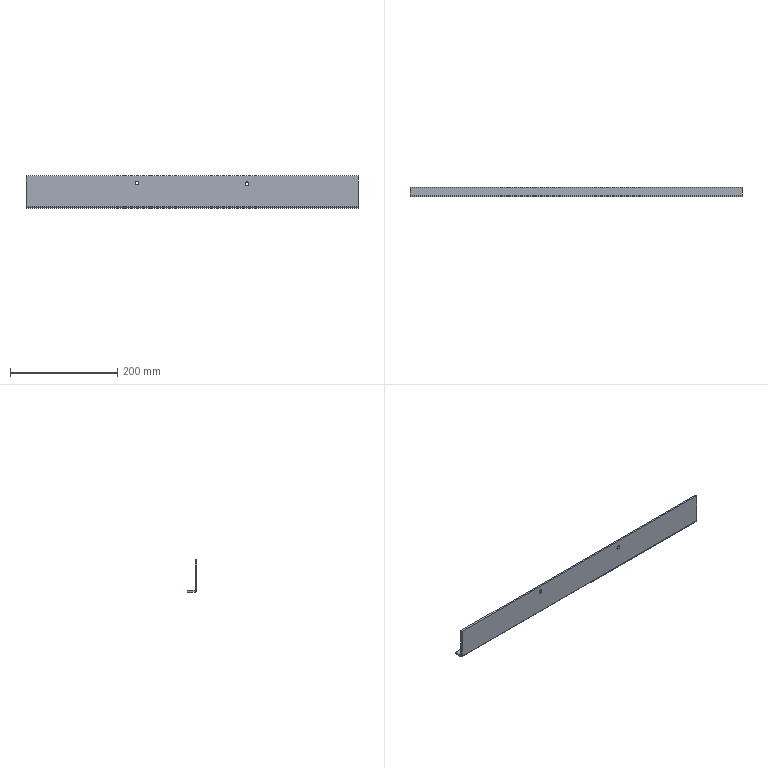Part | STEP file | HESS-408-70-15W-W-48-outer case reinforcing rib 7 | 1 solid | 14 faces | box 620 x 18 x 60 mm | volume 138005 mm3 | plane 8 | cylinder 6 | commonest cylinder face diameters 6.8 x4 0.2 x1 6.2 x1
STEP:
#1=CARTESIAN_POINT('',(0.,0.,0.));
#2=DIRECTION('',(0.,0.,1.));
#3=DIRECTION('',(1.,0.,0.));
#4=AXIS2_PLACEMENT_3D('',#1,#2,#3);
#5=CARTESIAN_POINT('',(102.5,0.,12.1));
#6=VERTEX_POINT('',#5);
#7=CARTESIAN_POINT('',(102.5,-3.,12.1));
#8=VERTEX_POINT('',#7);
#9=CARTESIAN_POINT('',(102.5,7.,12.1));
#10=DIRECTION('',(0.,-1.,0.));
#11=VECTOR('',#10,1.);
#12=LINE('',#9,#11);
#13=CARTESIAN_POINT('',(102.5,7.,15.5));
#14=DIRECTION('',(0.,-1.,0.));
#15=DIRECTION('',(0.,0.,-1.));
#16=AXIS2_PLACEMENT_3D('',#13,#14,#15);
#17=CYLINDRICAL_SURFACE('',#16,3.4);
#18=CARTESIAN_POINT('',(6.283,0.));
#19=DIRECTION('',(0.,1.));
#20=VECTOR('',#19,1.);
#21=LINE('',#18,#20);
#22=(GEOMETRIC_REPRESENTATION_CONTEXT(2)PARAMETRIC_REPRESENTATION_CONTEXT()REPRESENTATION_CONTEXT('',''));
#23=DEFINITIONAL_REPRESENTATION('',(#21),#22);
#24=PCURVE('',#17,#23);
#25=CARTESIAN_POINT('',(102.5,7.,15.5));
#26=DIRECTION('',(0.,-1.,0.));
#27=DIRECTION('',(0.,0.,-1.));
#28=AXIS2_PLACEMENT_3D('',#25,#26,#27);
#29=CYLINDRICAL_SURFACE('',#28,3.4);
#30=CARTESIAN_POINT('',(0.,0.));
#31=DIRECTION('',(0.,1.));
#32=VECTOR('',#31,1.);
#33=LINE('',#30,#32);
#34=(GEOMETRIC_REPRESENTATION_CONTEXT(2)PARAMETRIC_REPRESENTATION_CONTEXT()REPRESENTATION_CONTEXT('',''));
#35=DEFINITIONAL_REPRESENTATION('',(#33),#34);
#36=PCURVE('',#29,#35);
#37=SURFACE_CURVE('',#12,(#24,#36),.PCURVE_S1.);
#38=EDGE_CURVE('',#6,#8,#37,.T.);
#39=ORIENTED_EDGE('',*,*,#38,.T.);
#40=CARTESIAN_POINT('',(102.5,-3.,18.9));
#41=VERTEX_POINT('',#40);
#42=CARTESIAN_POINT('',(102.5,-3.,15.5));
#43=DIRECTION('',(0.,1.,0.));
#44=DIRECTION('',(0.,0.,-1.));
#45=AXIS2_PLACEMENT_3D('',#42,#43,#44);
#46=CIRCLE('',#45,3.4);
#47=CARTESIAN_POINT('',(6.283,10.));
#48=DIRECTION('',(-1.,0.));
#49=VECTOR('',#48,1.);
#50=LINE('',#47,#49);
#51=(GEOMETRIC_REPRESENTATION_CONTEXT(2)PARAMETRIC_REPRESENTATION_CONTEXT()REPRESENTATION_CONTEXT('',''));
#52=DEFINITIONAL_REPRESENTATION('',(#50),#51);
#53=PCURVE('',#17,#52);
#54=CARTESIAN_POINT('',(0.,-3.,0.));
#55=DIRECTION('',(0.,-1.,0.));
#56=DIRECTION('',(0.,0.,-1.));
#57=AXIS2_PLACEMENT_3D('',#54,#55,#56);
#58=PLANE('',#57);
#59=CARTESIAN_POINT('',(-12.1,102.5));
#60=CARTESIAN_POINT('',(-12.1,96.611));
#61=CARTESIAN_POINT('',(-17.2,99.556));
#62=CARTESIAN_POINT('',(-22.3,102.5));
#63=CARTESIAN_POINT('',(-17.2,105.444));
#64=CARTESIAN_POINT('',(-12.1,108.389));
#65=CARTESIAN_POINT('',(-12.1,102.5));
#66=(BOUNDED_CURVE()B_SPLINE_CURVE(2,(#59,#60,#61,#62,#63,#64,#65),.UNSPECIFIED.,.T.,.F.)B_SPLINE_CURVE_WITH_KNOTS((1,2,2,2,2,1),(-2.094,0.,2.094,4.189,6.283,8.378),.UNSPECIFIED.)CURVE()GEOMETRIC_REPRESENTATION_ITEM()RATIONAL_B_SPLINE_CURVE((1.,0.5,1.,0.5,1.,0.5,1.))REPRESENTATION_ITEM(''));
#67=(GEOMETRIC_REPRESENTATION_CONTEXT(2)PARAMETRIC_REPRESENTATION_CONTEXT()REPRESENTATION_CONTEXT('',''));
#68=DEFINITIONAL_REPRESENTATION('',(#66),#67);
#69=PCURVE('',#58,#68);
#70=SURFACE_CURVE('',#46,(#53,#69),.PCURVE_S1.);
#71=EDGE_CURVE('',#8,#41,#70,.T.);
#72=ORIENTED_EDGE('',*,*,#71,.T.);
#73=CARTESIAN_POINT('',(102.5,0.,18.9));
#74=VERTEX_POINT('',#73);
#75=CARTESIAN_POINT('',(102.5,7.,18.9));
#76=DIRECTION('',(0.,-1.,0.));
#77=VECTOR('',#76,1.);
#78=LINE('',#75,#77);
#79=CARTESIAN_POINT('',(3.142,0.));
#80=DIRECTION('',(0.,1.));
#81=VECTOR('',#80,1.);
#82=LINE('',#79,#81);
#83=(GEOMETRIC_REPRESENTATION_CONTEXT(2)PARAMETRIC_REPRESENTATION_CONTEXT()REPRESENTATION_CONTEXT('',''));
#84=DEFINITIONAL_REPRESENTATION('',(#82),#83);
#85=PCURVE('',#17,#84);
#86=CARTESIAN_POINT('',(3.142,0.));
#87=DIRECTION('',(0.,1.));
#88=VECTOR('',#87,1.);
#89=LINE('',#86,#88);
#90=(GEOMETRIC_REPRESENTATION_CONTEXT(2)PARAMETRIC_REPRESENTATION_CONTEXT()REPRESENTATION_CONTEXT('',''));
#91=DEFINITIONAL_REPRESENTATION('',(#89),#90);
#92=PCURVE('',#29,#91);
#93=SURFACE_CURVE('',#78,(#85,#92),.PCURVE_S1.);
#94=EDGE_CURVE('',#74,#41,#93,.T.);
#95=ORIENTED_EDGE('',*,*,#94,.F.);
#96=CARTESIAN_POINT('',(102.5,0.,15.5));
#97=DIRECTION('',(0.,-1.,0.));
#98=DIRECTION('',(0.,0.,-1.));
#99=AXIS2_PLACEMENT_3D('',#96,#97,#98);
#100=CIRCLE('',#99,3.4);
#101=CARTESIAN_POINT('',(0.,7.));
#102=DIRECTION('',(1.,0.));
#103=VECTOR('',#102,1.);
#104=LINE('',#101,#103);
#105=(GEOMETRIC_REPRESENTATION_CONTEXT(2)PARAMETRIC_REPRESENTATION_CONTEXT()REPRESENTATION_CONTEXT('',''));
#106=DEFINITIONAL_REPRESENTATION('',(#104),#105);
#107=PCURVE('',#17,#106);
#108=CARTESIAN_POINT('',(0.,0.,0.));
#109=DIRECTION('',(0.,-1.,0.));
#110=DIRECTION('',(0.,0.,-1.));
#111=AXIS2_PLACEMENT_3D('',#108,#109,#110);
#112=PLANE('',#111);
#113=CARTESIAN_POINT('',(-15.5,102.5));
#114=DIRECTION('',(1.,0.));
#115=AXIS2_PLACEMENT_2D('',#113,#114);
#116=CIRCLE('',#115,3.4);
#117=(GEOMETRIC_REPRESENTATION_CONTEXT(2)PARAMETRIC_REPRESENTATION_CONTEXT()REPRESENTATION_CONTEXT('',''));
#118=DEFINITIONAL_REPRESENTATION('',(#116),#117);
#119=PCURVE('',#112,#118);
#120=SURFACE_CURVE('',#100,(#107,#119),.PCURVE_S1.);
#121=EDGE_CURVE('',#74,#6,#120,.T.);
#122=ORIENTED_EDGE('',*,*,#121,.T.);
#123=EDGE_LOOP('',(#39,#72,#95,#122));
#124=FACE_BOUND('',#123,.F.);
#125=ADVANCED_FACE('',(#124),#17,.F.);
#126=CARTESIAN_POINT('',(-102.5,0.,13.6));
#127=VERTEX_POINT('',#126);
#128=CARTESIAN_POINT('',(-102.5,-3.,13.6));
#129=VERTEX_POINT('',#128);
#130=CARTESIAN_POINT('',(-102.5,7.,13.6));
#131=DIRECTION('',(0.,-1.,0.));
#132=VECTOR('',#131,1.);
#133=LINE('',#130,#132);
#134=CARTESIAN_POINT('',(-102.5,7.,17.));
#135=DIRECTION('',(0.,-1.,0.));
#136=DIRECTION('',(0.,0.,-1.));
#137=AXIS2_PLACEMENT_3D('',#134,#135,#136);
#138=CYLINDRICAL_SURFACE('',#137,3.4);
#139=CARTESIAN_POINT('',(6.283,0.));
#140=DIRECTION('',(0.,1.));
#141=VECTOR('',#140,1.);
#142=LINE('',#139,#141);
#143=(GEOMETRIC_REPRESENTATION_CONTEXT(2)PARAMETRIC_REPRESENTATION_CONTEXT()REPRESENTATION_CONTEXT('',''));
#144=DEFINITIONAL_REPRESENTATION('',(#142),#143);
#145=PCURVE('',#138,#144);
#146=CARTESIAN_POINT('',(-102.5,7.,17.));
#147=DIRECTION('',(0.,-1.,0.));
#148=DIRECTION('',(0.,0.,-1.));
#149=AXIS2_PLACEMENT_3D('',#146,#147,#148);
#150=CYLINDRICAL_SURFACE('',#149,3.4);
#151=CARTESIAN_POINT('',(0.,0.));
#152=DIRECTION('',(0.,1.));
#153=VECTOR('',#152,1.);
#154=LINE('',#151,#153);
#155=(GEOMETRIC_REPRESENTATION_CONTEXT(2)PARAMETRIC_REPRESENTATION_CONTEXT()REPRESENTATION_CONTEXT('',''));
#156=DEFINITIONAL_REPRESENTATION('',(#154),#155);
#157=PCURVE('',#150,#156);
#158=SURFACE_CURVE('',#133,(#145,#157),.PCURVE_S1.);
#159=EDGE_CURVE('',#127,#129,#158,.T.);
#160=ORIENTED_EDGE('',*,*,#159,.T.);
#161=CARTESIAN_POINT('',(-102.5,-3.,20.4));
#162=VERTEX_POINT('',#161);
#163=CARTESIAN_POINT('',(-102.5,-3.,17.));
#164=DIRECTION('',(0.,1.,0.));
#165=DIRECTION('',(0.,0.,-1.));
#166=AXIS2_PLACEMENT_3D('',#163,#164,#165);
#167=CIRCLE('',#166,3.4);
#168=CARTESIAN_POINT('',(6.283,10.));
#169=DIRECTION('',(-1.,0.));
#170=VECTOR('',#169,1.);
#171=LINE('',#168,#170);
#172=(GEOMETRIC_REPRESENTATION_CONTEXT(2)PARAMETRIC_REPRESENTATION_CONTEXT()REPRESENTATION_CONTEXT('',''));
#173=DEFINITIONAL_REPRESENTATION('',(#171),#172);
#174=PCURVE('',#138,#173);
#175=CARTESIAN_POINT('',(-13.6,-102.5));
#176=CARTESIAN_POINT('',(-13.6,-108.389));
#177=CARTESIAN_POINT('',(-18.7,-105.444));
#178=CARTESIAN_POINT('',(-23.8,-102.5));
#179=CARTESIAN_POINT('',(-18.7,-99.556));
#180=CARTESIAN_POINT('',(-13.6,-96.611));
#181=CARTESIAN_POINT('',(-13.6,-102.5));
#182=(BOUNDED_CURVE()B_SPLINE_CURVE(2,(#175,#176,#177,#178,#179,#180,#181),.UNSPECIFIED.,.T.,.F.)B_SPLINE_CURVE_WITH_KNOTS((1,2,2,2,2,1),(-2.094,0.,2.094,4.189,6.283,8.378),.UNSPECIFIED.)CURVE()GEOMETRIC_REPRESENTATION_ITEM()RATIONAL_B_SPLINE_CURVE((1.,0.5,1.,0.5,1.,0.5,1.))REPRESENTATION_ITEM(''));
#183=(GEOMETRIC_REPRESENTATION_CONTEXT(2)PARAMETRIC_REPRESENTATION_CONTEXT()REPRESENTATION_CONTEXT('',''));
#184=DEFINITIONAL_REPRESENTATION('',(#182),#183);
#185=PCURVE('',#58,#184);
#186=SURFACE_CURVE('',#167,(#174,#185),.PCURVE_S1.);
#187=EDGE_CURVE('',#129,#162,#186,.T.);
#188=ORIENTED_EDGE('',*,*,#187,.T.);
#189=CARTESIAN_POINT('',(-102.5,0.,20.4));
#190=VERTEX_POINT('',#189);
#191=CARTESIAN_POINT('',(-102.5,7.,20.4));
#192=DIRECTION('',(0.,-1.,0.));
#193=VECTOR('',#192,1.);
#194=LINE('',#191,#193);
#195=CARTESIAN_POINT('',(3.142,0.));
#196=DIRECTION('',(0.,1.));
#197=VECTOR('',#196,1.);
#198=LINE('',#195,#197);
#199=(GEOMETRIC_REPRESENTATION_CONTEXT(2)PARAMETRIC_REPRESENTATION_CONTEXT()REPRESENTATION_CONTEXT('',''));
#200=DEFINITIONAL_REPRESENTATION('',(#198),#199);
#201=PCURVE('',#138,#200);
#202=CARTESIAN_POINT('',(3.142,0.));
#203=DIRECTION('',(0.,1.));
#204=VECTOR('',#203,1.);
#205=LINE('',#202,#204);
#206=(GEOMETRIC_REPRESENTATION_CONTEXT(2)PARAMETRIC_REPRESENTATION_CONTEXT()REPRESENTATION_CONTEXT('',''));
#207=DEFINITIONAL_REPRESENTATION('',(#205),#206);
#208=PCURVE('',#150,#207);
#209=SURFACE_CURVE('',#194,(#201,#208),.PCURVE_S1.);
#210=EDGE_CURVE('',#190,#162,#209,.T.);
#211=ORIENTED_EDGE('',*,*,#210,.F.);
#212=CARTESIAN_POINT('',(-102.5,0.,17.));
#213=DIRECTION('',(0.,-1.,0.));
#214=DIRECTION('',(0.,0.,-1.));
#215=AXIS2_PLACEMENT_3D('',#212,#213,#214);
#216=CIRCLE('',#215,3.4);
#217=CARTESIAN_POINT('',(0.,7.));
#218=DIRECTION('',(1.,0.));
#219=VECTOR('',#218,1.);
#220=LINE('',#217,#219);
#221=(GEOMETRIC_REPRESENTATION_CONTEXT(2)PARAMETRIC_REPRESENTATION_CONTEXT()REPRESENTATION_CONTEXT('',''));
#222=DEFINITIONAL_REPRESENTATION('',(#220),#221);
#223=PCURVE('',#138,#222);
#224=CARTESIAN_POINT('',(-17.,-102.5));
#225=DIRECTION('',(1.,0.));
#226=AXIS2_PLACEMENT_2D('',#224,#225);
#227=CIRCLE('',#226,3.4);
#228=(GEOMETRIC_REPRESENTATION_CONTEXT(2)PARAMETRIC_REPRESENTATION_CONTEXT()REPRESENTATION_CONTEXT('',''));
#229=DEFINITIONAL_REPRESENTATION('',(#227),#228);
#230=PCURVE('',#112,#229);
#231=SURFACE_CURVE('',#216,(#223,#230),.PCURVE_S1.);
#232=EDGE_CURVE('',#190,#127,#231,.T.);
#233=ORIENTED_EDGE('',*,*,#232,.T.);
#234=EDGE_LOOP('',(#160,#188,#211,#233));
#235=FACE_BOUND('',#234,.F.);
#236=ADVANCED_FACE('',(#235),#138,.F.);
#237=CARTESIAN_POINT('',(310.,-3.,-26.9));
#238=VERTEX_POINT('',#237);
#239=CARTESIAN_POINT('',(310.,-3.,30.));
#240=VERTEX_POINT('',#239);
#241=CARTESIAN_POINT('',(310.,-3.,0.));
#242=DIRECTION('',(0.,0.,1.));
#243=VECTOR('',#242,1.);
#244=LINE('',#241,#243);
#245=CARTESIAN_POINT('',(0.,310.));
#246=DIRECTION('',(-1.,0.));
#247=VECTOR('',#246,1.);
#248=LINE('',#245,#247);
#249=(GEOMETRIC_REPRESENTATION_CONTEXT(2)PARAMETRIC_REPRESENTATION_CONTEXT()REPRESENTATION_CONTEXT('',''));
#250=DEFINITIONAL_REPRESENTATION('',(#248),#249);
#251=PCURVE('',#58,#250);
#252=CARTESIAN_POINT('',(310.,-3.,30.));
#253=DIRECTION('',(1.,0.,0.));
#254=DIRECTION('',(0.,0.,-1.));
#255=AXIS2_PLACEMENT_3D('',#252,#253,#254);
#256=PLANE('',#255);
#257=CARTESIAN_POINT('',(30.,0.));
#258=DIRECTION('',(-1.,0.));
#259=VECTOR('',#258,1.);
#260=LINE('',#257,#259);
#261=(GEOMETRIC_REPRESENTATION_CONTEXT(2)PARAMETRIC_REPRESENTATION_CONTEXT()REPRESENTATION_CONTEXT('',''));
#262=DEFINITIONAL_REPRESENTATION('',(#260),#261);
#263=PCURVE('',#256,#262);
#264=SURFACE_CURVE('',#244,(#251,#263),.PCURVE_S1.);
#265=EDGE_CURVE('',#238,#240,#264,.T.);
#266=ORIENTED_EDGE('',*,*,#265,.T.);
#267=CARTESIAN_POINT('',(-310.,-3.,30.));
#268=VERTEX_POINT('',#267);
#269=CARTESIAN_POINT('',(0.,-3.,30.));
#270=DIRECTION('',(-1.,0.,0.));
#271=VECTOR('',#270,1.);
#272=LINE('',#269,#271);
#273=CARTESIAN_POINT('',(-30.,0.));
#274=DIRECTION('',(0.,-1.));
#275=VECTOR('',#274,1.);
#276=LINE('',#273,#275);
#277=(GEOMETRIC_REPRESENTATION_CONTEXT(2)PARAMETRIC_REPRESENTATION_CONTEXT()REPRESENTATION_CONTEXT('',''));
#278=DEFINITIONAL_REPRESENTATION('',(#276),#277);
#279=PCURVE('',#58,#278);
#280=CARTESIAN_POINT('',(-310.,-3.,30.));
#281=DIRECTION('',(0.,0.,1.));
#282=DIRECTION('',(1.,0.,0.));
#283=AXIS2_PLACEMENT_3D('',#280,#281,#282);
#284=PLANE('',#283);
#285=CARTESIAN_POINT('',(310.,0.));
#286=DIRECTION('',(-1.,0.));
#287=VECTOR('',#286,1.);
#288=LINE('',#285,#287);
#289=(GEOMETRIC_REPRESENTATION_CONTEXT(2)PARAMETRIC_REPRESENTATION_CONTEXT()REPRESENTATION_CONTEXT('',''));
#290=DEFINITIONAL_REPRESENTATION('',(#288),#289);
#291=PCURVE('',#284,#290);
#292=SURFACE_CURVE('',#272,(#279,#291),.PCURVE_S1.);
#293=EDGE_CURVE('',#240,#268,#292,.T.);
#294=ORIENTED_EDGE('',*,*,#293,.T.);
#295=CARTESIAN_POINT('',(-310.,-3.,-26.9));
#296=VERTEX_POINT('',#295);
#297=CARTESIAN_POINT('',(-310.,-3.,0.));
#298=DIRECTION('',(0.,0.,-1.));
#299=VECTOR('',#298,1.);
#300=LINE('',#297,#299);
#301=CARTESIAN_POINT('',(0.,-310.));
#302=DIRECTION('',(1.,0.));
#303=VECTOR('',#302,1.);
#304=LINE('',#301,#303);
#305=(GEOMETRIC_REPRESENTATION_CONTEXT(2)PARAMETRIC_REPRESENTATION_CONTEXT()REPRESENTATION_CONTEXT('',''));
#306=DEFINITIONAL_REPRESENTATION('',(#304),#305);
#307=PCURVE('',#58,#306);
#308=CARTESIAN_POINT('',(-310.,-3.,30.));
#309=DIRECTION('',(-1.,0.,0.));
#310=DIRECTION('',(0.,0.,1.));
#311=AXIS2_PLACEMENT_3D('',#308,#309,#310);
#312=PLANE('',#311);
#313=CARTESIAN_POINT('',(-30.,0.));
#314=DIRECTION('',(-1.,0.));
#315=VECTOR('',#314,1.);
#316=LINE('',#313,#315);
#317=(GEOMETRIC_REPRESENTATION_CONTEXT(2)PARAMETRIC_REPRESENTATION_CONTEXT()REPRESENTATION_CONTEXT('',''));
#318=DEFINITIONAL_REPRESENTATION('',(#316),#317);
#319=PCURVE('',#312,#318);
#320=SURFACE_CURVE('',#300,(#307,#319),.PCURVE_S1.);
#321=EDGE_CURVE('',#268,#296,#320,.T.);
#322=ORIENTED_EDGE('',*,*,#321,.T.);
#323=CARTESIAN_POINT('',(0.,-3.,-26.9));
#324=DIRECTION('',(1.,0.,0.));
#325=VECTOR('',#324,1.);
#326=LINE('',#323,#325);
#327=CARTESIAN_POINT('',(26.9,0.));
#328=DIRECTION('',(0.,1.));
#329=VECTOR('',#328,1.);
#330=LINE('',#327,#329);
#331=(GEOMETRIC_REPRESENTATION_CONTEXT(2)PARAMETRIC_REPRESENTATION_CONTEXT()REPRESENTATION_CONTEXT('',''));
#332=DEFINITIONAL_REPRESENTATION('',(#330),#331);
#333=PCURVE('',#58,#332);
#334=CARTESIAN_POINT('',(-310.,0.1,-26.9));
#335=DIRECTION('',(-1.,0.,0.));
#336=DIRECTION('',(0.,-1.,0.));
#337=AXIS2_PLACEMENT_3D('',#334,#335,#336);
#338=CYLINDRICAL_SURFACE('',#337,3.1);
#339=CARTESIAN_POINT('',(6.283,-310.));
#340=DIRECTION('',(0.,-1.));
#341=VECTOR('',#340,1.);
#342=LINE('',#339,#341);
#343=(GEOMETRIC_REPRESENTATION_CONTEXT(2)PARAMETRIC_REPRESENTATION_CONTEXT()REPRESENTATION_CONTEXT('',''));
#344=DEFINITIONAL_REPRESENTATION('',(#342),#343);
#345=PCURVE('',#338,#344);
#346=SURFACE_CURVE('',#326,(#333,#345),.PCURVE_S1.);
#347=EDGE_CURVE('',#296,#238,#346,.T.);
#348=ORIENTED_EDGE('',*,*,#347,.T.);
#349=EDGE_LOOP('',(#266,#294,#322,#348));
#350=FACE_BOUND('',#349,.T.);
#351=ORIENTED_EDGE('',*,*,#71,.T.);
#352=CARTESIAN_POINT('',(102.5,-3.,15.5));
#353=DIRECTION('',(0.,1.,0.));
#354=DIRECTION('',(0.,0.,-1.));
#355=AXIS2_PLACEMENT_3D('',#352,#353,#354);
#356=CIRCLE('',#355,3.4);
#357=CARTESIAN_POINT('',(-12.1,102.5));
#358=CARTESIAN_POINT('',(-12.1,96.611));
#359=CARTESIAN_POINT('',(-17.2,99.556));
#360=CARTESIAN_POINT('',(-22.3,102.5));
#361=CARTESIAN_POINT('',(-17.2,105.444));
#362=CARTESIAN_POINT('',(-12.1,108.389));
#363=CARTESIAN_POINT('',(-12.1,102.5));
#364=(BOUNDED_CURVE()B_SPLINE_CURVE(2,(#357,#358,#359,#360,#361,#362,#363),.UNSPECIFIED.,.T.,.F.)B_SPLINE_CURVE_WITH_KNOTS((1,2,2,2,2,1),(-2.094,0.,2.094,4.189,6.283,8.378),.UNSPECIFIED.)CURVE()GEOMETRIC_REPRESENTATION_ITEM()RATIONAL_B_SPLINE_CURVE((1.,0.5,1.,0.5,1.,0.5,1.))REPRESENTATION_ITEM(''));
#365=(GEOMETRIC_REPRESENTATION_CONTEXT(2)PARAMETRIC_REPRESENTATION_CONTEXT()REPRESENTATION_CONTEXT('',''));
#366=DEFINITIONAL_REPRESENTATION('',(#364),#365);
#367=PCURVE('',#58,#366);
#368=CARTESIAN_POINT('',(6.283,10.));
#369=DIRECTION('',(-1.,0.));
#370=VECTOR('',#369,1.);
#371=LINE('',#368,#370);
#372=(GEOMETRIC_REPRESENTATION_CONTEXT(2)PARAMETRIC_REPRESENTATION_CONTEXT()REPRESENTATION_CONTEXT('',''));
#373=DEFINITIONAL_REPRESENTATION('',(#371),#372);
#374=PCURVE('',#29,#373);
#375=SURFACE_CURVE('',#356,(#367,#374),.PCURVE_S1.);
#376=EDGE_CURVE('',#41,#8,#375,.T.);
#377=ORIENTED_EDGE('',*,*,#376,.T.);
#378=EDGE_LOOP('',(#351,#377));
#379=FACE_BOUND('',#378,.T.);
#380=ORIENTED_EDGE('',*,*,#187,.T.);
#381=CARTESIAN_POINT('',(-102.5,-3.,17.));
#382=DIRECTION('',(0.,1.,0.));
#383=DIRECTION('',(0.,0.,-1.));
#384=AXIS2_PLACEMENT_3D('',#381,#382,#383);
#385=CIRCLE('',#384,3.4);
#386=CARTESIAN_POINT('',(-13.6,-102.5));
#387=CARTESIAN_POINT('',(-13.6,-108.389));
#388=CARTESIAN_POINT('',(-18.7,-105.444));
#389=CARTESIAN_POINT('',(-23.8,-102.5));
#390=CARTESIAN_POINT('',(-18.7,-99.556));
#391=CARTESIAN_POINT('',(-13.6,-96.611));
#392=CARTESIAN_POINT('',(-13.6,-102.5));
#393=(BOUNDED_CURVE()B_SPLINE_CURVE(2,(#386,#387,#388,#389,#390,#391,#392),.UNSPECIFIED.,.T.,.F.)B_SPLINE_CURVE_WITH_KNOTS((1,2,2,2,2,1),(-2.094,0.,2.094,4.189,6.283,8.378),.UNSPECIFIED.)CURVE()GEOMETRIC_REPRESENTATION_ITEM()RATIONAL_B_SPLINE_CURVE((1.,0.5,1.,0.5,1.,0.5,1.))REPRESENTATION_ITEM(''));
#394=(GEOMETRIC_REPRESENTATION_CONTEXT(2)PARAMETRIC_REPRESENTATION_CONTEXT()REPRESENTATION_CONTEXT('',''));
#395=DEFINITIONAL_REPRESENTATION('',(#393),#394);
#396=PCURVE('',#58,#395);
#397=CARTESIAN_POINT('',(6.283,10.));
#398=DIRECTION('',(-1.,0.));
#399=VECTOR('',#398,1.);
#400=LINE('',#397,#399);
#401=(GEOMETRIC_REPRESENTATION_CONTEXT(2)PARAMETRIC_REPRESENTATION_CONTEXT()REPRESENTATION_CONTEXT('',''));
#402=DEFINITIONAL_REPRESENTATION('',(#400),#401);
#403=PCURVE('',#150,#402);
#404=SURFACE_CURVE('',#385,(#396,#403),.PCURVE_S1.);
#405=EDGE_CURVE('',#162,#129,#404,.T.);
#406=ORIENTED_EDGE('',*,*,#405,.T.);
#407=EDGE_LOOP('',(#380,#406));
#408=FACE_BOUND('',#407,.T.);
#409=ADVANCED_FACE('',(#350,#379,#408),#58,.T.);
#410=ORIENTED_EDGE('',*,*,#293,.F.);
#411=CARTESIAN_POINT('',(310.,0.,30.));
#412=VERTEX_POINT('',#411);
#413=CARTESIAN_POINT('',(310.,-3.,30.));
#414=DIRECTION('',(0.,1.,0.));
#415=VECTOR('',#414,1.);
#416=LINE('',#413,#415);
#417=CARTESIAN_POINT('',(620.,0.));
#418=DIRECTION('',(0.,1.));
#419=VECTOR('',#418,1.);
#420=LINE('',#417,#419);
#421=(GEOMETRIC_REPRESENTATION_CONTEXT(2)PARAMETRIC_REPRESENTATION_CONTEXT()REPRESENTATION_CONTEXT('',''));
#422=DEFINITIONAL_REPRESENTATION('',(#420),#421);
#423=PCURVE('',#284,#422);
#424=CARTESIAN_POINT('',(0.,0.));
#425=DIRECTION('',(0.,1.));
#426=VECTOR('',#425,1.);
#427=LINE('',#424,#426);
#428=(GEOMETRIC_REPRESENTATION_CONTEXT(2)PARAMETRIC_REPRESENTATION_CONTEXT()REPRESENTATION_CONTEXT('',''));
#429=DEFINITIONAL_REPRESENTATION('',(#427),#428);
#430=PCURVE('',#256,#429);
#431=SURFACE_CURVE('',#416,(#423,#430),.PCURVE_S1.);
#432=EDGE_CURVE('',#240,#412,#431,.T.);
#433=ORIENTED_EDGE('',*,*,#432,.T.);
#434=CARTESIAN_POINT('',(-310.,0.,30.));
#435=VERTEX_POINT('',#434);
#436=CARTESIAN_POINT('',(-310.,0.,30.));
#437=DIRECTION('',(-1.,0.,0.));
#438=VECTOR('',#437,1.);
#439=LINE('',#436,#438);
#440=CARTESIAN_POINT('',(0.,3.));
#441=DIRECTION('',(-1.,0.));
#442=VECTOR('',#441,1.);
#443=LINE('',#440,#442);
#444=(GEOMETRIC_REPRESENTATION_CONTEXT(2)PARAMETRIC_REPRESENTATION_CONTEXT()REPRESENTATION_CONTEXT('',''));
#445=DEFINITIONAL_REPRESENTATION('',(#443),#444);
#446=PCURVE('',#284,#445);
#447=CARTESIAN_POINT('',(-30.,-310.));
#448=DIRECTION('',(0.,-1.));
#449=VECTOR('',#448,1.);
#450=LINE('',#447,#449);
#451=(GEOMETRIC_REPRESENTATION_CONTEXT(2)PARAMETRIC_REPRESENTATION_CONTEXT()REPRESENTATION_CONTEXT('',''));
#452=DEFINITIONAL_REPRESENTATION('',(#450),#451);
#453=PCURVE('',#112,#452);
#454=SURFACE_CURVE('',#439,(#446,#453),.PCURVE_S1.);
#455=EDGE_CURVE('',#412,#435,#454,.T.);
#456=ORIENTED_EDGE('',*,*,#455,.T.);
#457=CARTESIAN_POINT('',(-310.,-3.,30.));
#458=DIRECTION('',(0.,-1.,0.));
#459=VECTOR('',#458,1.);
#460=LINE('',#457,#459);
#461=CARTESIAN_POINT('',(0.,0.));
#462=DIRECTION('',(0.,-1.));
#463=VECTOR('',#462,1.);
#464=LINE('',#461,#463);
#465=(GEOMETRIC_REPRESENTATION_CONTEXT(2)PARAMETRIC_REPRESENTATION_CONTEXT()REPRESENTATION_CONTEXT('',''));
#466=DEFINITIONAL_REPRESENTATION('',(#464),#465);
#467=PCURVE('',#284,#466);
#468=CARTESIAN_POINT('',(0.,0.));
#469=DIRECTION('',(0.,-1.));
#470=VECTOR('',#469,1.);
#471=LINE('',#468,#470);
#472=(GEOMETRIC_REPRESENTATION_CONTEXT(2)PARAMETRIC_REPRESENTATION_CONTEXT()REPRESENTATION_CONTEXT('',''));
#473=DEFINITIONAL_REPRESENTATION('',(#471),#472);
#474=PCURVE('',#312,#473);
#475=SURFACE_CURVE('',#460,(#467,#474),.PCURVE_S1.);
#476=EDGE_CURVE('',#435,#268,#475,.T.);
#477=ORIENTED_EDGE('',*,*,#476,.T.);
#478=EDGE_LOOP('',(#410,#433,#456,#477));
#479=FACE_BOUND('',#478,.T.);
#480=ADVANCED_FACE('',(#479),#284,.T.);
#481=ORIENTED_EDGE('',*,*,#432,.F.);
#482=ORIENTED_EDGE('',*,*,#265,.F.);
#483=CARTESIAN_POINT('',(310.,0.1,-30.));
#484=VERTEX_POINT('',#483);
#485=CARTESIAN_POINT('',(310.,0.1,-26.9));
#486=DIRECTION('',(-1.,0.,0.));
#487=DIRECTION('',(0.,-1.,0.));
#488=AXIS2_PLACEMENT_3D('',#485,#486,#487);
#489=CIRCLE('',#488,3.1);
#490=CARTESIAN_POINT('',(56.9,0.));
#491=CARTESIAN_POINT('',(51.531,0.));
#492=CARTESIAN_POINT('',(54.215,4.65));
#493=CARTESIAN_POINT('',(56.9,9.3));
#494=CARTESIAN_POINT('',(59.585,4.65));
#495=CARTESIAN_POINT('',(62.269,0.));
#496=CARTESIAN_POINT('',(56.9,0.));
#497=(BOUNDED_CURVE()B_SPLINE_CURVE(2,(#490,#491,#492,#493,#494,#495,#496),.UNSPECIFIED.,.T.,.F.)B_SPLINE_CURVE_WITH_KNOTS((1,2,2,2,2,1),(-2.094,0.,2.094,4.189,6.283,8.378),.UNSPECIFIED.)CURVE()GEOMETRIC_REPRESENTATION_ITEM()RATIONAL_B_SPLINE_CURVE((1.,0.5,1.,0.5,1.,0.5,1.))REPRESENTATION_ITEM(''));
#498=(GEOMETRIC_REPRESENTATION_CONTEXT(2)PARAMETRIC_REPRESENTATION_CONTEXT()REPRESENTATION_CONTEXT('',''));
#499=DEFINITIONAL_REPRESENTATION('',(#497),#498);
#500=PCURVE('',#256,#499);
#501=CARTESIAN_POINT('',(0.,-620.));
#502=DIRECTION('',(1.,0.));
#503=VECTOR('',#502,1.);
#504=LINE('',#501,#503);
#505=(GEOMETRIC_REPRESENTATION_CONTEXT(2)PARAMETRIC_REPRESENTATION_CONTEXT()REPRESENTATION_CONTEXT('',''));
#506=DEFINITIONAL_REPRESENTATION('',(#504),#505);
#507=PCURVE('',#338,#506);
#508=SURFACE_CURVE('',#489,(#500,#507),.PCURVE_S1.);
#509=EDGE_CURVE('',#484,#238,#508,.T.);
#510=ORIENTED_EDGE('',*,*,#509,.F.);
#511=CARTESIAN_POINT('',(310.,15.,-30.));
#512=VERTEX_POINT('',#511);
#513=CARTESIAN_POINT('',(310.,0.,-30.));
#514=DIRECTION('',(0.,1.,0.));
#515=VECTOR('',#514,1.);
#516=LINE('',#513,#515);
#517=CARTESIAN_POINT('',(60.,3.));
#518=DIRECTION('',(0.,1.));
#519=VECTOR('',#518,1.);
#520=LINE('',#517,#519);
#521=(GEOMETRIC_REPRESENTATION_CONTEXT(2)PARAMETRIC_REPRESENTATION_CONTEXT()REPRESENTATION_CONTEXT('',''));
#522=DEFINITIONAL_REPRESENTATION('',(#520),#521);
#523=PCURVE('',#256,#522);
#524=CARTESIAN_POINT('',(0.,0.,-30.));
#525=DIRECTION('',(0.,0.,1.));
#526=DIRECTION('',(0.,-1.,0.));
#527=AXIS2_PLACEMENT_3D('',#524,#525,#526);
#528=PLANE('',#527);
#529=CARTESIAN_POINT('',(0.,310.));
#530=DIRECTION('',(-1.,0.));
#531=VECTOR('',#530,1.);
#532=LINE('',#529,#531);
#533=(GEOMETRIC_REPRESENTATION_CONTEXT(2)PARAMETRIC_REPRESENTATION_CONTEXT()REPRESENTATION_CONTEXT('',''));
#534=DEFINITIONAL_REPRESENTATION('',(#532),#533);
#535=PCURVE('',#528,#534);
#536=SURFACE_CURVE('',#516,(#523,#535),.PCURVE_S1.);
#537=EDGE_CURVE('',#484,#512,#536,.T.);
#538=ORIENTED_EDGE('',*,*,#537,.T.);
#539=CARTESIAN_POINT('',(310.,15.,-27.));
#540=VERTEX_POINT('',#539);
#541=CARTESIAN_POINT('',(310.,15.,-30.));
#542=DIRECTION('',(0.,0.,-1.));
#543=VECTOR('',#542,1.);
#544=LINE('',#541,#543);
#545=CARTESIAN_POINT('',(60.,18.));
#546=DIRECTION('',(1.,0.));
#547=VECTOR('',#546,1.);
#548=LINE('',#545,#547);
#549=(GEOMETRIC_REPRESENTATION_CONTEXT(2)PARAMETRIC_REPRESENTATION_CONTEXT()REPRESENTATION_CONTEXT('',''));
#550=DEFINITIONAL_REPRESENTATION('',(#548),#549);
#551=PCURVE('',#256,#550);
#552=CARTESIAN_POINT('',(310.,15.,-30.));
#553=DIRECTION('',(0.,-1.,0.));
#554=DIRECTION('',(0.,0.,-1.));
#555=AXIS2_PLACEMENT_3D('',#552,#553,#554);
#556=PLANE('',#555);
#557=CARTESIAN_POINT('',(0.,0.));
#558=DIRECTION('',(1.,0.));
#559=VECTOR('',#558,1.);
#560=LINE('',#557,#559);
#561=(GEOMETRIC_REPRESENTATION_CONTEXT(2)PARAMETRIC_REPRESENTATION_CONTEXT()REPRESENTATION_CONTEXT('',''));
#562=DEFINITIONAL_REPRESENTATION('',(#560),#561);
#563=PCURVE('',#556,#562);
#564=SURFACE_CURVE('',#544,(#551,#563),.PCURVE_S1.);
#565=EDGE_CURVE('',#540,#512,#564,.T.);
#566=ORIENTED_EDGE('',*,*,#565,.F.);
#567=CARTESIAN_POINT('',(310.,0.1,-27.));
#568=VERTEX_POINT('',#567);
#569=CARTESIAN_POINT('',(310.,0.,-27.));
#570=DIRECTION('',(0.,1.,0.));
#571=VECTOR('',#570,1.);
#572=LINE('',#569,#571);
#573=CARTESIAN_POINT('',(57.,3.));
#574=DIRECTION('',(0.,1.));
#575=VECTOR('',#574,1.);
#576=LINE('',#573,#575);
#577=(GEOMETRIC_REPRESENTATION_CONTEXT(2)PARAMETRIC_REPRESENTATION_CONTEXT()REPRESENTATION_CONTEXT('',''));
#578=DEFINITIONAL_REPRESENTATION('',(#576),#577);
#579=PCURVE('',#256,#578);
#580=CARTESIAN_POINT('',(0.,0.,-27.));
#581=DIRECTION('',(0.,0.,1.));
#582=DIRECTION('',(0.,-1.,0.));
#583=AXIS2_PLACEMENT_3D('',#580,#581,#582);
#584=PLANE('',#583);
#585=CARTESIAN_POINT('',(0.,310.));
#586=DIRECTION('',(-1.,0.));
#587=VECTOR('',#586,1.);
#588=LINE('',#585,#587);
#589=(GEOMETRIC_REPRESENTATION_CONTEXT(2)PARAMETRIC_REPRESENTATION_CONTEXT()REPRESENTATION_CONTEXT('',''));
#590=DEFINITIONAL_REPRESENTATION('',(#588),#589);
#591=PCURVE('',#584,#590);
#592=SURFACE_CURVE('',#572,(#579,#591),.PCURVE_S1.);
#593=EDGE_CURVE('',#568,#540,#592,.T.);
#594=ORIENTED_EDGE('',*,*,#593,.F.);
#595=CARTESIAN_POINT('',(310.,0.,-26.9));
#596=VERTEX_POINT('',#595);
#597=CARTESIAN_POINT('',(310.,0.1,-26.9));
#598=DIRECTION('',(-1.,0.,0.));
#599=DIRECTION('',(0.,-1.,0.));
#600=AXIS2_PLACEMENT_3D('',#597,#598,#599);
#601=CIRCLE('',#600,0.1);
#602=CARTESIAN_POINT('',(56.9,3.));
#603=CARTESIAN_POINT('',(56.727,3.));
#604=CARTESIAN_POINT('',(56.813,3.15));
#605=CARTESIAN_POINT('',(56.9,3.3));
#606=CARTESIAN_POINT('',(56.987,3.15));
#607=CARTESIAN_POINT('',(57.073,3.));
#608=CARTESIAN_POINT('',(56.9,3.));
#609=(BOUNDED_CURVE()B_SPLINE_CURVE(2,(#602,#603,#604,#605,#606,#607,#608),.UNSPECIFIED.,.T.,.F.)B_SPLINE_CURVE_WITH_KNOTS((1,2,2,2,2,1),(-2.094,0.,2.094,4.189,6.283,8.378),.UNSPECIFIED.)CURVE()GEOMETRIC_REPRESENTATION_ITEM()RATIONAL_B_SPLINE_CURVE((1.,0.5,1.,0.5,1.,0.5,1.))REPRESENTATION_ITEM(''));
#610=(GEOMETRIC_REPRESENTATION_CONTEXT(2)PARAMETRIC_REPRESENTATION_CONTEXT()REPRESENTATION_CONTEXT('',''));
#611=DEFINITIONAL_REPRESENTATION('',(#609),#610);
#612=PCURVE('',#256,#611);
#613=CARTESIAN_POINT('',(-310.,0.1,-26.9));
#614=DIRECTION('',(-1.,0.,0.));
#615=DIRECTION('',(0.,-1.,0.));
#616=AXIS2_PLACEMENT_3D('',#613,#614,#615);
#617=CYLINDRICAL_SURFACE('',#616,0.1);
#618=CARTESIAN_POINT('',(0.,-620.));
#619=DIRECTION('',(1.,0.));
#620=VECTOR('',#619,1.);
#621=LINE('',#618,#620);
#622=(GEOMETRIC_REPRESENTATION_CONTEXT(2)PARAMETRIC_REPRESENTATION_CONTEXT()REPRESENTATION_CONTEXT('',''));
#623=DEFINITIONAL_REPRESENTATION('',(#621),#622);
#624=PCURVE('',#617,#623);
#625=SURFACE_CURVE('',#601,(#612,#624),.PCURVE_S1.);
#626=EDGE_CURVE('',#568,#596,#625,.T.);
#627=ORIENTED_EDGE('',*,*,#626,.T.);
#628=CARTESIAN_POINT('',(310.,0.,30.));
#629=DIRECTION('',(0.,0.,1.));
#630=VECTOR('',#629,1.);
#631=LINE('',#628,#630);
#632=CARTESIAN_POINT('',(0.,3.));
#633=DIRECTION('',(-1.,0.));
#634=VECTOR('',#633,1.);
#635=LINE('',#632,#634);
#636=(GEOMETRIC_REPRESENTATION_CONTEXT(2)PARAMETRIC_REPRESENTATION_CONTEXT()REPRESENTATION_CONTEXT('',''));
#637=DEFINITIONAL_REPRESENTATION('',(#635),#636);
#638=PCURVE('',#256,#637);
#639=CARTESIAN_POINT('',(-30.,310.));
#640=DIRECTION('',(-1.,0.));
#641=VECTOR('',#640,1.);
#642=LINE('',#639,#641);
#643=(GEOMETRIC_REPRESENTATION_CONTEXT(2)PARAMETRIC_REPRESENTATION_CONTEXT()REPRESENTATION_CONTEXT('',''));
#644=DEFINITIONAL_REPRESENTATION('',(#642),#643);
#645=PCURVE('',#112,#644);
#646=SURFACE_CURVE('',#631,(#638,#645),.PCURVE_S1.);
#647=EDGE_CURVE('',#596,#412,#646,.T.);
#648=ORIENTED_EDGE('',*,*,#647,.T.);
#649=EDGE_LOOP('',(#481,#482,#510,#538,#566,#594,#627,#648));
#650=FACE_BOUND('',#649,.T.);
#651=ADVANCED_FACE('',(#650),#256,.T.);
#652=CARTESIAN_POINT('',(-310.,0.1,-30.));
#653=VERTEX_POINT('',#652);
#654=CARTESIAN_POINT('',(-310.,0.1,-30.));
#655=DIRECTION('',(1.,0.,0.));
#656=VECTOR('',#655,1.);
#657=LINE('',#654,#656);
#658=CARTESIAN_POINT('',(4.712,0.));
#659=DIRECTION('',(0.,-1.));
#660=VECTOR('',#659,1.);
#661=LINE('',#658,#660);
#662=(GEOMETRIC_REPRESENTATION_CONTEXT(2)PARAMETRIC_REPRESENTATION_CONTEXT()REPRESENTATION_CONTEXT('',''));
#663=DEFINITIONAL_REPRESENTATION('',(#661),#662);
#664=PCURVE('',#338,#663);
#665=CARTESIAN_POINT('',(-0.1,-310.));
#666=DIRECTION('',(0.,1.));
#667=VECTOR('',#666,1.);
#668=LINE('',#665,#667);
#669=(GEOMETRIC_REPRESENTATION_CONTEXT(2)PARAMETRIC_REPRESENTATION_CONTEXT()REPRESENTATION_CONTEXT('',''));
#670=DEFINITIONAL_REPRESENTATION('',(#668),#669);
#671=PCURVE('',#528,#670);
#672=SURFACE_CURVE('',#657,(#664,#671),.PCURVE_S1.);
#673=EDGE_CURVE('',#653,#484,#672,.T.);
#674=ORIENTED_EDGE('',*,*,#673,.T.);
#675=ORIENTED_EDGE('',*,*,#509,.T.);
#676=ORIENTED_EDGE('',*,*,#347,.F.);
#677=CARTESIAN_POINT('',(-310.,0.1,-26.9));
#678=DIRECTION('',(1.,0.,0.));
#679=DIRECTION('',(0.,-1.,0.));
#680=AXIS2_PLACEMENT_3D('',#677,#678,#679);
#681=CIRCLE('',#680,3.1);
#682=CARTESIAN_POINT('',(6.283,0.));
#683=DIRECTION('',(-1.,0.));
#684=VECTOR('',#683,1.);
#685=LINE('',#682,#684);
#686=(GEOMETRIC_REPRESENTATION_CONTEXT(2)PARAMETRIC_REPRESENTATION_CONTEXT()REPRESENTATION_CONTEXT('',''));
#687=DEFINITIONAL_REPRESENTATION('',(#685),#686);
#688=PCURVE('',#338,#687);
#689=CARTESIAN_POINT('',(-56.9,0.));
#690=CARTESIAN_POINT('',(-62.269,0.));
#691=CARTESIAN_POINT('',(-59.585,4.65));
#692=CARTESIAN_POINT('',(-56.9,9.3));
#693=CARTESIAN_POINT('',(-54.215,4.65));
#694=CARTESIAN_POINT('',(-51.531,0.));
#695=CARTESIAN_POINT('',(-56.9,0.));
#696=(BOUNDED_CURVE()B_SPLINE_CURVE(2,(#689,#690,#691,#692,#693,#694,#695),.UNSPECIFIED.,.T.,.F.)B_SPLINE_CURVE_WITH_KNOTS((1,2,2,2,2,1),(-2.094,0.,2.094,4.189,6.283,8.378),.UNSPECIFIED.)CURVE()GEOMETRIC_REPRESENTATION_ITEM()RATIONAL_B_SPLINE_CURVE((1.,0.5,1.,0.5,1.,0.5,1.))REPRESENTATION_ITEM(''));
#697=(GEOMETRIC_REPRESENTATION_CONTEXT(2)PARAMETRIC_REPRESENTATION_CONTEXT()REPRESENTATION_CONTEXT('',''));
#698=DEFINITIONAL_REPRESENTATION('',(#696),#697);
#699=PCURVE('',#312,#698);
#700=SURFACE_CURVE('',#681,(#688,#699),.PCURVE_S1.);
#701=EDGE_CURVE('',#296,#653,#700,.T.);
#702=ORIENTED_EDGE('',*,*,#701,.T.);
#703=EDGE_LOOP('',(#674,#675,#676,#702));
#704=FACE_BOUND('',#703,.T.);
#705=ADVANCED_FACE('',(#704),#338,.T.);
#706=ORIENTED_EDGE('',*,*,#321,.F.);
#707=ORIENTED_EDGE('',*,*,#476,.F.);
#708=CARTESIAN_POINT('',(-310.,0.,-26.9));
#709=VERTEX_POINT('',#708);
#710=CARTESIAN_POINT('',(-310.,0.,30.));
#711=DIRECTION('',(0.,0.,-1.));
#712=VECTOR('',#711,1.);
#713=LINE('',#710,#712);
#714=CARTESIAN_POINT('',(0.,3.));
#715=DIRECTION('',(-1.,0.));
#716=VECTOR('',#715,1.);
#717=LINE('',#714,#716);
#718=(GEOMETRIC_REPRESENTATION_CONTEXT(2)PARAMETRIC_REPRESENTATION_CONTEXT()REPRESENTATION_CONTEXT('',''));
#719=DEFINITIONAL_REPRESENTATION('',(#717),#718);
#720=PCURVE('',#312,#719);
#721=CARTESIAN_POINT('',(-30.,-310.));
#722=DIRECTION('',(1.,0.));
#723=VECTOR('',#722,1.);
#724=LINE('',#721,#723);
#725=(GEOMETRIC_REPRESENTATION_CONTEXT(2)PARAMETRIC_REPRESENTATION_CONTEXT()REPRESENTATION_CONTEXT('',''));
#726=DEFINITIONAL_REPRESENTATION('',(#724),#725);
#727=PCURVE('',#112,#726);
#728=SURFACE_CURVE('',#713,(#720,#727),.PCURVE_S1.);
#729=EDGE_CURVE('',#435,#709,#728,.T.);
#730=ORIENTED_EDGE('',*,*,#729,.T.);
#731=CARTESIAN_POINT('',(-310.,0.1,-27.));
#732=VERTEX_POINT('',#731);
#733=CARTESIAN_POINT('',(-310.,0.1,-26.9));
#734=DIRECTION('',(-1.,0.,0.));
#735=DIRECTION('',(0.,-1.,0.));
#736=AXIS2_PLACEMENT_3D('',#733,#734,#735);
#737=CIRCLE('',#736,0.1);
#738=CARTESIAN_POINT('',(-56.9,3.1));
#739=DIRECTION('',(0.,-1.));
#740=AXIS2_PLACEMENT_2D('',#738,#739);
#741=CIRCLE('',#740,0.1);
#742=(GEOMETRIC_REPRESENTATION_CONTEXT(2)PARAMETRIC_REPRESENTATION_CONTEXT()REPRESENTATION_CONTEXT('',''));
#743=DEFINITIONAL_REPRESENTATION('',(#741),#742);
#744=PCURVE('',#312,#743);
#745=CARTESIAN_POINT('',(0.,0.));
#746=DIRECTION('',(1.,0.));
#747=VECTOR('',#746,1.);
#748=LINE('',#745,#747);
#749=(GEOMETRIC_REPRESENTATION_CONTEXT(2)PARAMETRIC_REPRESENTATION_CONTEXT()REPRESENTATION_CONTEXT('',''));
#750=DEFINITIONAL_REPRESENTATION('',(#748),#749);
#751=PCURVE('',#617,#750);
#752=SURFACE_CURVE('',#737,(#744,#751),.PCURVE_S1.);
#753=EDGE_CURVE('',#732,#709,#752,.T.);
#754=ORIENTED_EDGE('',*,*,#753,.F.);
#755=CARTESIAN_POINT('',(-310.,15.,-27.));
#756=VERTEX_POINT('',#755);
#757=CARTESIAN_POINT('',(-310.,15.,-27.));
#758=DIRECTION('',(0.,-1.,0.));
#759=VECTOR('',#758,1.);
#760=LINE('',#757,#759);
#761=CARTESIAN_POINT('',(-57.,18.));
#762=DIRECTION('',(0.,-1.));
#763=VECTOR('',#762,1.);
#764=LINE('',#761,#763);
#765=(GEOMETRIC_REPRESENTATION_CONTEXT(2)PARAMETRIC_REPRESENTATION_CONTEXT()REPRESENTATION_CONTEXT('',''));
#766=DEFINITIONAL_REPRESENTATION('',(#764),#765);
#767=PCURVE('',#312,#766);
#768=CARTESIAN_POINT('',(-15.,-310.));
#769=DIRECTION('',(1.,0.));
#770=VECTOR('',#769,1.);
#771=LINE('',#768,#770);
#772=(GEOMETRIC_REPRESENTATION_CONTEXT(2)PARAMETRIC_REPRESENTATION_CONTEXT()REPRESENTATION_CONTEXT('',''));
#773=DEFINITIONAL_REPRESENTATION('',(#771),#772);
#774=PCURVE('',#584,#773);
#775=SURFACE_CURVE('',#760,(#767,#774),.PCURVE_S1.);
#776=EDGE_CURVE('',#756,#732,#775,.T.);
#777=ORIENTED_EDGE('',*,*,#776,.F.);
#778=CARTESIAN_POINT('',(-310.,15.,-30.));
#779=VERTEX_POINT('',#778);
#780=CARTESIAN_POINT('',(-310.,15.,-30.));
#781=DIRECTION('',(0.,0.,1.));
#782=VECTOR('',#781,1.);
#783=LINE('',#780,#782);
#784=CARTESIAN_POINT('',(-60.,18.));
#785=DIRECTION('',(1.,0.));
#786=VECTOR('',#785,1.);
#787=LINE('',#784,#786);
#788=(GEOMETRIC_REPRESENTATION_CONTEXT(2)PARAMETRIC_REPRESENTATION_CONTEXT()REPRESENTATION_CONTEXT('',''));
#789=DEFINITIONAL_REPRESENTATION('',(#787),#788);
#790=PCURVE('',#312,#789);
#791=CARTESIAN_POINT('',(0.,-620.));
#792=DIRECTION('',(-1.,0.));
#793=VECTOR('',#792,1.);
#794=LINE('',#791,#793);
#795=(GEOMETRIC_REPRESENTATION_CONTEXT(2)PARAMETRIC_REPRESENTATION_CONTEXT()REPRESENTATION_CONTEXT('',''));
#796=DEFINITIONAL_REPRESENTATION('',(#794),#795);
#797=PCURVE('',#556,#796);
#798=SURFACE_CURVE('',#783,(#790,#797),.PCURVE_S1.);
#799=EDGE_CURVE('',#779,#756,#798,.T.);
#800=ORIENTED_EDGE('',*,*,#799,.F.);
#801=CARTESIAN_POINT('',(-310.,0.,-30.));
#802=DIRECTION('',(0.,-1.,0.));
#803=VECTOR('',#802,1.);
#804=LINE('',#801,#803);
#805=CARTESIAN_POINT('',(-60.,3.));
#806=DIRECTION('',(0.,-1.));
#807=VECTOR('',#806,1.);
#808=LINE('',#805,#807);
#809=(GEOMETRIC_REPRESENTATION_CONTEXT(2)PARAMETRIC_REPRESENTATION_CONTEXT()REPRESENTATION_CONTEXT('',''));
#810=DEFINITIONAL_REPRESENTATION('',(#808),#809);
#811=PCURVE('',#312,#810);
#812=CARTESIAN_POINT('',(0.,-310.));
#813=DIRECTION('',(1.,0.));
#814=VECTOR('',#813,1.);
#815=LINE('',#812,#814);
#816=(GEOMETRIC_REPRESENTATION_CONTEXT(2)PARAMETRIC_REPRESENTATION_CONTEXT()REPRESENTATION_CONTEXT('',''));
#817=DEFINITIONAL_REPRESENTATION('',(#815),#816);
#818=PCURVE('',#528,#817);
#819=SURFACE_CURVE('',#804,(#811,#818),.PCURVE_S1.);
#820=EDGE_CURVE('',#779,#653,#819,.T.);
#821=ORIENTED_EDGE('',*,*,#820,.T.);
#822=ORIENTED_EDGE('',*,*,#701,.F.);
#823=EDGE_LOOP('',(#706,#707,#730,#754,#777,#800,#821,#822));
#824=FACE_BOUND('',#823,.T.);
#825=ADVANCED_FACE('',(#824),#312,.T.);
#826=ORIENTED_EDGE('',*,*,#376,.T.);
#827=ORIENTED_EDGE('',*,*,#38,.F.);
#828=CARTESIAN_POINT('',(102.5,0.,15.5));
#829=DIRECTION('',(0.,-1.,0.));
#830=DIRECTION('',(0.,0.,-1.));
#831=AXIS2_PLACEMENT_3D('',#828,#829,#830);
#832=CIRCLE('',#831,3.4);
#833=CARTESIAN_POINT('',(0.,7.));
#834=DIRECTION('',(1.,0.));
#835=VECTOR('',#834,1.);
#836=LINE('',#833,#835);
#837=(GEOMETRIC_REPRESENTATION_CONTEXT(2)PARAMETRIC_REPRESENTATION_CONTEXT()REPRESENTATION_CONTEXT('',''));
#838=DEFINITIONAL_REPRESENTATION('',(#836),#837);
#839=PCURVE('',#29,#838);
#840=CARTESIAN_POINT('',(-15.5,102.5));
#841=DIRECTION('',(1.,0.));
#842=AXIS2_PLACEMENT_2D('',#840,#841);
#843=CIRCLE('',#842,3.4);
#844=(GEOMETRIC_REPRESENTATION_CONTEXT(2)PARAMETRIC_REPRESENTATION_CONTEXT()REPRESENTATION_CONTEXT('',''));
#845=DEFINITIONAL_REPRESENTATION('',(#843),#844);
#846=PCURVE('',#112,#845);
#847=SURFACE_CURVE('',#832,(#839,#846),.PCURVE_S1.);
#848=EDGE_CURVE('',#6,#74,#847,.T.);
#849=ORIENTED_EDGE('',*,*,#848,.T.);
#850=ORIENTED_EDGE('',*,*,#94,.T.);
#851=EDGE_LOOP('',(#826,#827,#849,#850));
#852=FACE_BOUND('',#851,.F.);
#853=ADVANCED_FACE('',(#852),#29,.F.);
#854=ORIENTED_EDGE('',*,*,#405,.T.);
#855=ORIENTED_EDGE('',*,*,#159,.F.);
#856=CARTESIAN_POINT('',(-102.5,0.,17.));
#857=DIRECTION('',(0.,-1.,0.));
#858=DIRECTION('',(0.,0.,-1.));
#859=AXIS2_PLACEMENT_3D('',#856,#857,#858);
#860=CIRCLE('',#859,3.4);
#861=CARTESIAN_POINT('',(0.,7.));
#862=DIRECTION('',(1.,0.));
#863=VECTOR('',#862,1.);
#864=LINE('',#861,#863);
#865=(GEOMETRIC_REPRESENTATION_CONTEXT(2)PARAMETRIC_REPRESENTATION_CONTEXT()REPRESENTATION_CONTEXT('',''));
#866=DEFINITIONAL_REPRESENTATION('',(#864),#865);
#867=PCURVE('',#150,#866);
#868=CARTESIAN_POINT('',(-17.,-102.5));
#869=DIRECTION('',(1.,0.));
#870=AXIS2_PLACEMENT_2D('',#868,#869);
#871=CIRCLE('',#870,3.4);
#872=(GEOMETRIC_REPRESENTATION_CONTEXT(2)PARAMETRIC_REPRESENTATION_CONTEXT()REPRESENTATION_CONTEXT('',''));
#873=DEFINITIONAL_REPRESENTATION('',(#871),#872);
#874=PCURVE('',#112,#873);
#875=SURFACE_CURVE('',#860,(#867,#874),.PCURVE_S1.);
#876=EDGE_CURVE('',#127,#190,#875,.T.);
#877=ORIENTED_EDGE('',*,*,#876,.T.);
#878=ORIENTED_EDGE('',*,*,#210,.T.);
#879=EDGE_LOOP('',(#854,#855,#877,#878));
#880=FACE_BOUND('',#879,.F.);
#881=ADVANCED_FACE('',(#880),#150,.F.);
#882=ORIENTED_EDGE('',*,*,#729,.F.);
#883=ORIENTED_EDGE('',*,*,#455,.F.);
#884=ORIENTED_EDGE('',*,*,#647,.F.);
#885=CARTESIAN_POINT('',(0.,0.,-26.9));
#886=DIRECTION('',(1.,0.,0.));
#887=VECTOR('',#886,1.);
#888=LINE('',#885,#887);
#889=CARTESIAN_POINT('',(26.9,0.));
#890=DIRECTION('',(0.,1.));
#891=VECTOR('',#890,1.);
#892=LINE('',#889,#891);
#893=(GEOMETRIC_REPRESENTATION_CONTEXT(2)PARAMETRIC_REPRESENTATION_CONTEXT()REPRESENTATION_CONTEXT('',''));
#894=DEFINITIONAL_REPRESENTATION('',(#892),#893);
#895=PCURVE('',#112,#894);
#896=CARTESIAN_POINT('',(6.283,-310.));
#897=DIRECTION('',(0.,-1.));
#898=VECTOR('',#897,1.);
#899=LINE('',#896,#898);
#900=(GEOMETRIC_REPRESENTATION_CONTEXT(2)PARAMETRIC_REPRESENTATION_CONTEXT()REPRESENTATION_CONTEXT('',''));
#901=DEFINITIONAL_REPRESENTATION('',(#899),#900);
#902=PCURVE('',#617,#901);
#903=SURFACE_CURVE('',#888,(#895,#902),.PCURVE_S1.);
#904=EDGE_CURVE('',#709,#596,#903,.T.);
#905=ORIENTED_EDGE('',*,*,#904,.F.);
#906=EDGE_LOOP('',(#882,#883,#884,#905));
#907=FACE_BOUND('',#906,.T.);
#908=ORIENTED_EDGE('',*,*,#848,.T.);
#909=ORIENTED_EDGE('',*,*,#121,.T.);
#910=EDGE_LOOP('',(#908,#909));
#911=FACE_BOUND('',#910,.T.);
#912=ORIENTED_EDGE('',*,*,#876,.T.);
#913=ORIENTED_EDGE('',*,*,#232,.T.);
#914=EDGE_LOOP('',(#912,#913));
#915=FACE_BOUND('',#914,.T.);
#916=ADVANCED_FACE('',(#907,#911,#915),#112,.F.);
#917=ORIENTED_EDGE('',*,*,#820,.F.);
#918=CARTESIAN_POINT('',(0.,15.,-30.));
#919=DIRECTION('',(-1.,0.,0.));
#920=VECTOR('',#919,1.);
#921=LINE('',#918,#920);
#922=CARTESIAN_POINT('',(-15.,0.));
#923=DIRECTION('',(0.,-1.));
#924=VECTOR('',#923,1.);
#925=LINE('',#922,#924);
#926=(GEOMETRIC_REPRESENTATION_CONTEXT(2)PARAMETRIC_REPRESENTATION_CONTEXT()REPRESENTATION_CONTEXT('',''));
#927=DEFINITIONAL_REPRESENTATION('',(#925),#926);
#928=PCURVE('',#528,#927);
#929=CARTESIAN_POINT('',(0.,-310.));
#930=DIRECTION('',(0.,-1.));
#931=VECTOR('',#930,1.);
#932=LINE('',#929,#931);
#933=(GEOMETRIC_REPRESENTATION_CONTEXT(2)PARAMETRIC_REPRESENTATION_CONTEXT()REPRESENTATION_CONTEXT('',''));
#934=DEFINITIONAL_REPRESENTATION('',(#932),#933);
#935=PCURVE('',#556,#934);
#936=SURFACE_CURVE('',#921,(#928,#935),.PCURVE_S1.);
#937=EDGE_CURVE('',#512,#779,#936,.T.);
#938=ORIENTED_EDGE('',*,*,#937,.F.);
#939=ORIENTED_EDGE('',*,*,#537,.F.);
#940=ORIENTED_EDGE('',*,*,#673,.F.);
#941=EDGE_LOOP('',(#917,#938,#939,#940));
#942=FACE_BOUND('',#941,.T.);
#943=ADVANCED_FACE('',(#942),#528,.F.);
#944=ORIENTED_EDGE('',*,*,#904,.F.);
#945=ORIENTED_EDGE('',*,*,#753,.F.);
#946=CARTESIAN_POINT('',(-310.,0.1,-27.));
#947=DIRECTION('',(1.,0.,0.));
#948=VECTOR('',#947,1.);
#949=LINE('',#946,#948);
#950=CARTESIAN_POINT('',(4.712,0.));
#951=DIRECTION('',(0.,-1.));
#952=VECTOR('',#951,1.);
#953=LINE('',#950,#952);
#954=(GEOMETRIC_REPRESENTATION_CONTEXT(2)PARAMETRIC_REPRESENTATION_CONTEXT()REPRESENTATION_CONTEXT('',''));
#955=DEFINITIONAL_REPRESENTATION('',(#953),#954);
#956=PCURVE('',#617,#955);
#957=CARTESIAN_POINT('',(-0.1,-310.));
#958=DIRECTION('',(0.,1.));
#959=VECTOR('',#958,1.);
#960=LINE('',#957,#959);
#961=(GEOMETRIC_REPRESENTATION_CONTEXT(2)PARAMETRIC_REPRESENTATION_CONTEXT()REPRESENTATION_CONTEXT('',''));
#962=DEFINITIONAL_REPRESENTATION('',(#960),#961);
#963=PCURVE('',#584,#962);
#964=SURFACE_CURVE('',#949,(#956,#963),.PCURVE_S1.);
#965=EDGE_CURVE('',#732,#568,#964,.T.);
#966=ORIENTED_EDGE('',*,*,#965,.T.);
#967=ORIENTED_EDGE('',*,*,#626,.T.);
#968=EDGE_LOOP('',(#944,#945,#966,#967));
#969=FACE_BOUND('',#968,.F.);
#970=ADVANCED_FACE('',(#969),#617,.F.);
#971=ORIENTED_EDGE('',*,*,#565,.T.);
#972=ORIENTED_EDGE('',*,*,#937,.T.);
#973=ORIENTED_EDGE('',*,*,#799,.T.);
#974=CARTESIAN_POINT('',(310.,15.,-27.));
#975=DIRECTION('',(-1.,0.,0.));
#976=VECTOR('',#975,1.);
#977=LINE('',#974,#976);
#978=CARTESIAN_POINT('',(-3.,0.));
#979=DIRECTION('',(0.,-1.));
#980=VECTOR('',#979,1.);
#981=LINE('',#978,#980);
#982=(GEOMETRIC_REPRESENTATION_CONTEXT(2)PARAMETRIC_REPRESENTATION_CONTEXT()REPRESENTATION_CONTEXT('',''));
#983=DEFINITIONAL_REPRESENTATION('',(#981),#982);
#984=PCURVE('',#556,#983);
#985=CARTESIAN_POINT('',(-15.,310.));
#986=DIRECTION('',(0.,-1.));
#987=VECTOR('',#986,1.);
#988=LINE('',#985,#987);
#989=(GEOMETRIC_REPRESENTATION_CONTEXT(2)PARAMETRIC_REPRESENTATION_CONTEXT()REPRESENTATION_CONTEXT('',''));
#990=DEFINITIONAL_REPRESENTATION('',(#988),#989);
#991=PCURVE('',#584,#990);
#992=SURFACE_CURVE('',#977,(#984,#991),.PCURVE_S1.);
#993=EDGE_CURVE('',#540,#756,#992,.T.);
#994=ORIENTED_EDGE('',*,*,#993,.F.);
#995=EDGE_LOOP('',(#971,#972,#973,#994));
#996=FACE_BOUND('',#995,.T.);
#997=ADVANCED_FACE('',(#996),#556,.F.);
#998=ORIENTED_EDGE('',*,*,#593,.T.);
#999=ORIENTED_EDGE('',*,*,#993,.T.);
#1000=ORIENTED_EDGE('',*,*,#776,.T.);
#1001=ORIENTED_EDGE('',*,*,#965,.T.);
#1002=EDGE_LOOP('',(#998,#999,#1000,#1001));
#1003=FACE_BOUND('',#1002,.T.);
#1004=ADVANCED_FACE('',(#1003),#584,.T.);
#1005=CLOSED_SHELL('',(#125,#236,#409,#480,#651,#705,#825,#853,#881,#916,#943,#970,#997,#1004));
#1006=MANIFOLD_SOLID_BREP('',#1005);
#1007=(LENGTH_UNIT()NAMED_UNIT(*)SI_UNIT(.MILLI.,.METRE.));
#1008=UNCERTAINTY_MEASURE_WITH_UNIT(LENGTH_MEASURE(0.0000001),#1007,'','');
#1009=(NAMED_UNIT(*)PLANE_ANGLE_UNIT()SI_UNIT($,.RADIAN.));
#1010=(NAMED_UNIT(*)SI_UNIT($,.STERADIAN.)SOLID_ANGLE_UNIT());
#1011=(GEOMETRIC_REPRESENTATION_CONTEXT(3)GLOBAL_UNCERTAINTY_ASSIGNED_CONTEXT((#1008))GLOBAL_UNIT_ASSIGNED_CONTEXT((#1007,#1009,#1010))REPRESENTATION_CONTEXT('',''));
#1012=ADVANCED_BREP_SHAPE_REPRESENTATION('',(#4,#1006),#1011);